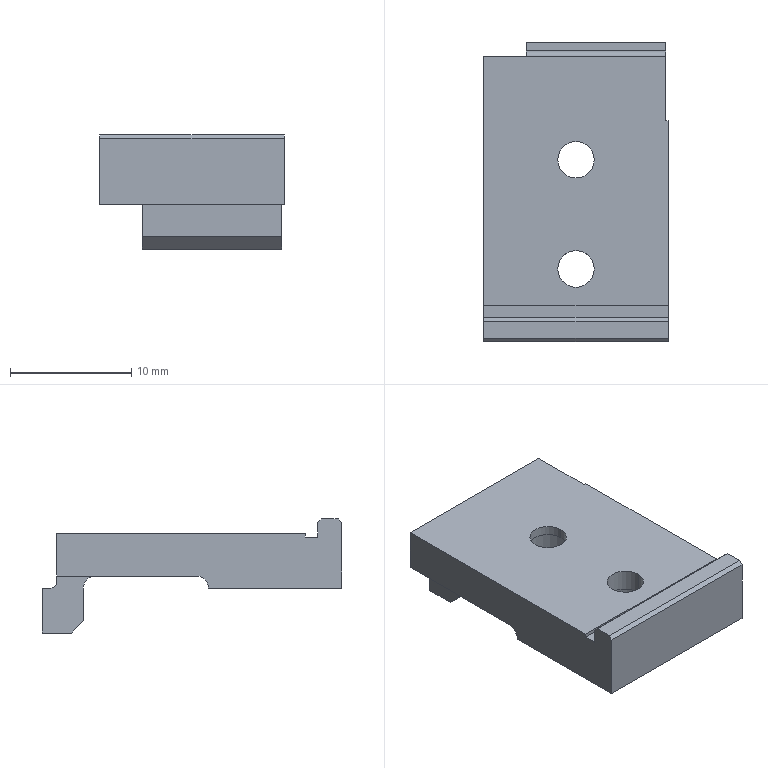Part | NX | 1 solid | 34 faces | box 15.2 x 24.7 x 9.4 mm | volume 1490 mm3 | plane 23 | cylinder 11 | commonest cylinder face diameters 3 x4 5 x4 2 x2 1 x1
STEP:
#1=CARTESIAN_POINT('',(-15.2,-12.7,1.));
#2=VERTEX_POINT('',#1);
#3=CARTESIAN_POINT('',(-15.2,-1.2,1.));
#4=VERTEX_POINT('',#3);
#5=CARTESIAN_POINT('',(-15.2,0.,1.));
#6=DIRECTION('',(0.,1.,0.));
#7=VECTOR('',#6,1000.);
#8=LINE('',#5,#7);
#9=EDGE_CURVE('',#2,#4,#8,.T.);
#10=ORIENTED_EDGE('',*,*,#9,.F.);
#11=CARTESIAN_POINT('',(-15.2,-13.7,0.));
#12=VERTEX_POINT('',#11);
#13=CARTESIAN_POINT('',(-15.2,-12.7,0.));
#14=DIRECTION('',(1.,0.,0.));
#15=DIRECTION('',(0.,-1.,0.));
#16=AXIS2_PLACEMENT_3D('',#13,#14,#15);
#17=CIRCLE('',#16,1.);
#18=EDGE_CURVE('',#2,#12,#17,.T.);
#19=ORIENTED_EDGE('',*,*,#18,.T.);
#20=CARTESIAN_POINT('',(-15.2,-24.7,0.));
#21=VERTEX_POINT('',#20);
#22=CARTESIAN_POINT('',(-15.2,0.,0.));
#23=DIRECTION('',(0.,1.,0.));
#24=VECTOR('',#23,1000.);
#25=LINE('',#22,#24);
#26=EDGE_CURVE('',#21,#12,#25,.T.);
#27=ORIENTED_EDGE('',*,*,#26,.F.);
#28=CARTESIAN_POINT('',(-15.2,-24.7,5.4));
#29=VERTEX_POINT('',#28);
#30=CARTESIAN_POINT('',(-15.2,-24.7,0.));
#31=DIRECTION('',(0.,0.,-1.));
#32=VECTOR('',#31,1000.);
#33=LINE('',#30,#32);
#34=EDGE_CURVE('',#29,#21,#33,.T.);
#35=ORIENTED_EDGE('',*,*,#34,.F.);
#36=CARTESIAN_POINT('',(-15.2,-24.4,5.7));
#37=VERTEX_POINT('',#36);
#38=CARTESIAN_POINT('',(-15.2,0.,30.1));
#39=DIRECTION('',(0.,0.7071,0.7071));
#40=VECTOR('',#39,1000.);
#41=LINE('',#38,#40);
#42=EDGE_CURVE('',#29,#37,#41,.T.);
#43=ORIENTED_EDGE('',*,*,#42,.T.);
#44=CARTESIAN_POINT('',(-15.2,-23.,5.7));
#45=VERTEX_POINT('',#44);
#46=CARTESIAN_POINT('',(-15.2,0.,5.7));
#47=DIRECTION('',(0.,1.,0.));
#48=VECTOR('',#47,1000.);
#49=LINE('',#46,#48);
#50=EDGE_CURVE('',#37,#45,#49,.T.);
#51=ORIENTED_EDGE('',*,*,#50,.T.);
#52=CARTESIAN_POINT('',(-15.2,-22.7,5.4));
#53=VERTEX_POINT('',#52);
#54=CARTESIAN_POINT('',(-15.2,0.,-17.3));
#55=DIRECTION('',(0.,-0.7071,0.7071));
#56=VECTOR('',#55,1000.);
#57=LINE('',#54,#56);
#58=EDGE_CURVE('',#53,#45,#57,.T.);
#59=ORIENTED_EDGE('',*,*,#58,.F.);
#60=CARTESIAN_POINT('',(-15.2,-22.7,4.2));
#61=VERTEX_POINT('',#60);
#62=CARTESIAN_POINT('',(-15.2,-22.7,0.));
#63=DIRECTION('',(0.,0.,-1.));
#64=VECTOR('',#63,1000.);
#65=LINE('',#62,#64);
#66=EDGE_CURVE('',#53,#61,#65,.T.);
#67=ORIENTED_EDGE('',*,*,#66,.T.);
#68=CARTESIAN_POINT('',(-15.2,-21.7,4.2));
#69=VERTEX_POINT('',#68);
#70=CARTESIAN_POINT('',(-15.2,0.,4.2));
#71=DIRECTION('',(0.,-1.,0.));
#72=VECTOR('',#71,1000.);
#73=LINE('',#70,#72);
#74=EDGE_CURVE('',#69,#61,#73,.T.);
#75=ORIENTED_EDGE('',*,*,#74,.F.);
#76=CARTESIAN_POINT('',(-15.2,-21.7,4.5));
#77=VERTEX_POINT('',#76);
#78=CARTESIAN_POINT('',(-15.2,-21.7,0.));
#79=DIRECTION('',(0.,0.,-1.));
#80=VECTOR('',#79,1000.);
#81=LINE('',#78,#80);
#82=EDGE_CURVE('',#77,#69,#81,.T.);
#83=ORIENTED_EDGE('',*,*,#82,.F.);
#84=CARTESIAN_POINT('',(-15.2,-1.2,4.5));
#85=VERTEX_POINT('',#84);
#86=CARTESIAN_POINT('',(-15.2,0.,4.5));
#87=DIRECTION('',(0.,-1.,0.));
#88=VECTOR('',#87,1000.);
#89=LINE('',#86,#88);
#90=EDGE_CURVE('',#85,#77,#89,.T.);
#91=ORIENTED_EDGE('',*,*,#90,.F.);
#92=CARTESIAN_POINT('',(-15.2,-1.2,0.));
#93=DIRECTION('',(0.,0.,1.));
#94=VECTOR('',#93,1000.);
#95=LINE('',#92,#94);
#96=EDGE_CURVE('',#4,#85,#95,.T.);
#97=ORIENTED_EDGE('',*,*,#96,.F.);
#98=EDGE_LOOP('',(#10,#19,#27,#35,#43,#51,#59,#67,#75,#83,#91,#97));
#99=FACE_BOUND('',#98,.T.);
#100=CARTESIAN_POINT('',(-15.2,0.,0.));
#101=DIRECTION('',(1.,0.,0.));
#102=DIRECTION('',(0.,1.,0.));
#103=AXIS2_PLACEMENT_3D('',#100,#101,#102);
#104=PLANE('',#103);
#105=ADVANCED_FACE('',(#99),#104,.F.);
#106=CARTESIAN_POINT('',(0.,-21.7,4.5));
#107=VERTEX_POINT('',#106);
#108=CARTESIAN_POINT('',(0.,-6.5,4.5));
#109=VERTEX_POINT('',#108);
#110=CARTESIAN_POINT('',(0.,0.,4.5));
#111=DIRECTION('',(0.,1.,0.));
#112=VECTOR('',#111,1000.);
#113=LINE('',#110,#112);
#114=EDGE_CURVE('',#107,#109,#113,.T.);
#115=ORIENTED_EDGE('',*,*,#114,.F.);
#116=CARTESIAN_POINT('',(0.,-21.7,4.2));
#117=VERTEX_POINT('',#116);
#118=CARTESIAN_POINT('',(0.,-21.7,0.));
#119=DIRECTION('',(0.,0.,1.));
#120=VECTOR('',#119,1000.);
#121=LINE('',#118,#120);
#122=EDGE_CURVE('',#117,#107,#121,.T.);
#123=ORIENTED_EDGE('',*,*,#122,.F.);
#124=CARTESIAN_POINT('',(0.,-22.7,4.2));
#125=VERTEX_POINT('',#124);
#126=CARTESIAN_POINT('',(0.,0.,4.2));
#127=DIRECTION('',(0.,1.,0.));
#128=VECTOR('',#127,1000.);
#129=LINE('',#126,#128);
#130=EDGE_CURVE('',#125,#117,#129,.T.);
#131=ORIENTED_EDGE('',*,*,#130,.F.);
#132=CARTESIAN_POINT('',(0.,-22.7,5.4));
#133=VERTEX_POINT('',#132);
#134=CARTESIAN_POINT('',(0.,-22.7,0.));
#135=DIRECTION('',(0.,0.,1.));
#136=VECTOR('',#135,1000.);
#137=LINE('',#134,#136);
#138=EDGE_CURVE('',#125,#133,#137,.T.);
#139=ORIENTED_EDGE('',*,*,#138,.T.);
#140=CARTESIAN_POINT('',(0.,-23.,5.7));
#141=VERTEX_POINT('',#140);
#142=CARTESIAN_POINT('',(0.,0.,-17.3));
#143=DIRECTION('',(0.,0.7071,-0.7071));
#144=VECTOR('',#143,1000.);
#145=LINE('',#142,#144);
#146=EDGE_CURVE('',#141,#133,#145,.T.);
#147=ORIENTED_EDGE('',*,*,#146,.F.);
#148=CARTESIAN_POINT('',(0.,-24.4,5.7));
#149=VERTEX_POINT('',#148);
#150=CARTESIAN_POINT('',(0.,0.,5.7));
#151=DIRECTION('',(0.,-1.,0.));
#152=VECTOR('',#151,1000.);
#153=LINE('',#150,#152);
#154=EDGE_CURVE('',#141,#149,#153,.T.);
#155=ORIENTED_EDGE('',*,*,#154,.T.);
#156=CARTESIAN_POINT('',(0.,-24.7,5.4));
#157=VERTEX_POINT('',#156);
#158=CARTESIAN_POINT('',(0.,0.,30.1));
#159=DIRECTION('',(0.,-0.7071,-0.7071));
#160=VECTOR('',#159,1000.);
#161=LINE('',#158,#160);
#162=EDGE_CURVE('',#149,#157,#161,.T.);
#163=ORIENTED_EDGE('',*,*,#162,.T.);
#164=CARTESIAN_POINT('',(0.,-24.7,0.));
#165=VERTEX_POINT('',#164);
#166=CARTESIAN_POINT('',(0.,-24.7,0.));
#167=DIRECTION('',(0.,0.,1.));
#168=VECTOR('',#167,1000.);
#169=LINE('',#166,#168);
#170=EDGE_CURVE('',#165,#157,#169,.T.);
#171=ORIENTED_EDGE('',*,*,#170,.F.);
#172=CARTESIAN_POINT('',(0.,-13.7,0.));
#173=VERTEX_POINT('',#172);
#174=CARTESIAN_POINT('',(0.,0.,0.));
#175=DIRECTION('',(0.,-1.,0.));
#176=VECTOR('',#175,1000.);
#177=LINE('',#174,#176);
#178=EDGE_CURVE('',#173,#165,#177,.T.);
#179=ORIENTED_EDGE('',*,*,#178,.F.);
#180=CARTESIAN_POINT('',(0.,-12.7,1.));
#181=VERTEX_POINT('',#180);
#182=CARTESIAN_POINT('',(0.,-12.7,0.));
#183=DIRECTION('',(1.,0.,0.));
#184=DIRECTION('',(0.,-1.,0.));
#185=AXIS2_PLACEMENT_3D('',#182,#183,#184);
#186=CIRCLE('',#185,1.);
#187=EDGE_CURVE('',#181,#173,#186,.T.);
#188=ORIENTED_EDGE('',*,*,#187,.F.);
#189=CARTESIAN_POINT('',(0.,-6.5,1.));
#190=VERTEX_POINT('',#189);
#191=CARTESIAN_POINT('',(0.,0.,1.));
#192=DIRECTION('',(0.,-1.,0.));
#193=VECTOR('',#192,1000.);
#194=LINE('',#191,#193);
#195=EDGE_CURVE('',#190,#181,#194,.T.);
#196=ORIENTED_EDGE('',*,*,#195,.F.);
#197=CARTESIAN_POINT('',(0.,-6.5,0.));
#198=DIRECTION('',(0.,0.,-1.));
#199=VECTOR('',#198,1000.);
#200=LINE('',#197,#199);
#201=EDGE_CURVE('',#109,#190,#200,.T.);
#202=ORIENTED_EDGE('',*,*,#201,.F.);
#203=EDGE_LOOP('',(#115,#123,#131,#139,#147,#155,#163,#171,#179,#188,#196,#202));
#204=FACE_BOUND('',#203,.T.);
#205=CARTESIAN_POINT('',(0.,-24.7,0.));
#206=DIRECTION('',(-1.,0.,0.));
#207=DIRECTION('',(0.,0.,1.));
#208=AXIS2_PLACEMENT_3D('',#205,#206,#207);
#209=PLANE('',#208);
#210=ADVANCED_FACE('',(#204),#209,.F.);
#211=CARTESIAN_POINT('',(-5.1,-18.7,2.7));
#212=VERTEX_POINT('',#211);
#213=CARTESIAN_POINT('',(-10.1,-18.7,2.7));
#214=VERTEX_POINT('',#213);
#215=CARTESIAN_POINT('',(-7.6,-18.7,2.7));
#216=DIRECTION('',(0.,0.,-1.));
#217=DIRECTION('',(-1.,0.,0.));
#218=AXIS2_PLACEMENT_3D('',#215,#216,#217);
#219=CIRCLE('',#218,2.5);
#220=EDGE_CURVE('',#212,#214,#219,.T.);
#221=ORIENTED_EDGE('',*,*,#220,.T.);
#222=CARTESIAN_POINT('',(-7.6,-18.7,2.7));
#223=DIRECTION('',(0.,0.,-1.));
#224=DIRECTION('',(-1.,0.,0.));
#225=AXIS2_PLACEMENT_3D('',#222,#223,#224);
#226=CIRCLE('',#225,2.5);
#227=EDGE_CURVE('',#214,#212,#226,.T.);
#228=ORIENTED_EDGE('',*,*,#227,.T.);
#229=EDGE_LOOP('',(#221,#228));
#230=FACE_BOUND('',#229,.T.);
#231=CARTESIAN_POINT('',(-9.1,-18.7,2.7));
#232=VERTEX_POINT('',#231);
#233=CARTESIAN_POINT('',(-6.1,-18.7,2.7));
#234=VERTEX_POINT('',#233);
#235=CARTESIAN_POINT('',(-7.6,-18.7,2.7));
#236=DIRECTION('',(0.,0.,-1.));
#237=DIRECTION('',(-1.,0.,0.));
#238=AXIS2_PLACEMENT_3D('',#235,#236,#237);
#239=CIRCLE('',#238,1.5);
#240=EDGE_CURVE('',#232,#234,#239,.T.);
#241=ORIENTED_EDGE('',*,*,#240,.F.);
#242=CARTESIAN_POINT('',(-7.6,-18.7,2.7));
#243=DIRECTION('',(0.,0.,-1.));
#244=DIRECTION('',(-1.,0.,0.));
#245=AXIS2_PLACEMENT_3D('',#242,#243,#244);
#246=CIRCLE('',#245,1.5);
#247=EDGE_CURVE('',#234,#232,#246,.T.);
#248=ORIENTED_EDGE('',*,*,#247,.F.);
#249=EDGE_LOOP('',(#241,#248));
#250=FACE_BOUND('',#249,.T.);
#251=CARTESIAN_POINT('',(-11.486,-5.492,2.7));
#252=DIRECTION('',(0.,0.,-1.));
#253=DIRECTION('',(0.,-1.,0.));
#254=AXIS2_PLACEMENT_3D('',#251,#252,#253);
#255=PLANE('',#254);
#256=ADVANCED_FACE('',(#230,#250),#255,.T.);
#257=CARTESIAN_POINT('',(-0.2,-1.2,4.5));
#258=VERTEX_POINT('',#257);
#259=CARTESIAN_POINT('',(-0.2,-6.5,4.5));
#260=VERTEX_POINT('',#259);
#261=CARTESIAN_POINT('',(-0.2,0.,4.5));
#262=DIRECTION('',(0.,-1.,0.));
#263=VECTOR('',#262,1000.);
#264=LINE('',#261,#263);
#265=EDGE_CURVE('',#258,#260,#264,.T.);
#266=ORIENTED_EDGE('',*,*,#265,.F.);
#267=CARTESIAN_POINT('',(0.,-1.2,4.5));
#268=DIRECTION('',(1.,0.,0.));
#269=VECTOR('',#268,1000.);
#270=LINE('',#267,#269);
#271=EDGE_CURVE('',#85,#258,#270,.T.);
#272=ORIENTED_EDGE('',*,*,#271,.F.);
#273=ORIENTED_EDGE('',*,*,#90,.T.);
#274=CARTESIAN_POINT('',(0.,-21.7,4.5));
#275=DIRECTION('',(-1.,0.,0.));
#276=VECTOR('',#275,1000.);
#277=LINE('',#274,#276);
#278=EDGE_CURVE('',#107,#77,#277,.T.);
#279=ORIENTED_EDGE('',*,*,#278,.F.);
#280=ORIENTED_EDGE('',*,*,#114,.T.);
#281=CARTESIAN_POINT('',(0.,-6.5,4.5));
#282=DIRECTION('',(1.,0.,0.));
#283=VECTOR('',#282,1000.);
#284=LINE('',#281,#283);
#285=EDGE_CURVE('',#260,#109,#284,.T.);
#286=ORIENTED_EDGE('',*,*,#285,.F.);
#287=EDGE_LOOP('',(#266,#272,#273,#279,#280,#286));
#288=FACE_BOUND('',#287,.T.);
#289=CARTESIAN_POINT('',(-6.1,-9.7,4.5));
#290=VERTEX_POINT('',#289);
#291=CARTESIAN_POINT('',(-9.1,-9.7,4.5));
#292=VERTEX_POINT('',#291);
#293=CARTESIAN_POINT('',(-7.6,-9.7,4.5));
#294=DIRECTION('',(0.,0.,-1.));
#295=DIRECTION('',(-1.,0.,0.));
#296=AXIS2_PLACEMENT_3D('',#293,#294,#295);
#297=CIRCLE('',#296,1.5);
#298=EDGE_CURVE('',#290,#292,#297,.T.);
#299=ORIENTED_EDGE('',*,*,#298,.T.);
#300=CARTESIAN_POINT('',(-7.6,-9.7,4.5));
#301=DIRECTION('',(0.,0.,-1.));
#302=DIRECTION('',(-1.,0.,0.));
#303=AXIS2_PLACEMENT_3D('',#300,#301,#302);
#304=CIRCLE('',#303,1.5);
#305=EDGE_CURVE('',#292,#290,#304,.T.);
#306=ORIENTED_EDGE('',*,*,#305,.T.);
#307=EDGE_LOOP('',(#299,#306));
#308=FACE_BOUND('',#307,.T.);
#309=CARTESIAN_POINT('',(-9.1,-18.7,4.5));
#310=VERTEX_POINT('',#309);
#311=CARTESIAN_POINT('',(-6.1,-18.7,4.5));
#312=VERTEX_POINT('',#311);
#313=CARTESIAN_POINT('',(-7.6,-18.7,4.5));
#314=DIRECTION('',(0.,0.,-1.));
#315=DIRECTION('',(-1.,0.,0.));
#316=AXIS2_PLACEMENT_3D('',#313,#314,#315);
#317=CIRCLE('',#316,1.5);
#318=EDGE_CURVE('',#310,#312,#317,.T.);
#319=ORIENTED_EDGE('',*,*,#318,.T.);
#320=CARTESIAN_POINT('',(-7.6,-18.7,4.5));
#321=DIRECTION('',(0.,0.,-1.));
#322=DIRECTION('',(-1.,0.,0.));
#323=AXIS2_PLACEMENT_3D('',#320,#321,#322);
#324=CIRCLE('',#323,1.5);
#325=EDGE_CURVE('',#312,#310,#324,.T.);
#326=ORIENTED_EDGE('',*,*,#325,.T.);
#327=EDGE_LOOP('',(#319,#326));
#328=FACE_BOUND('',#327,.T.);
#329=CARTESIAN_POINT('',(0.,0.,4.5));
#330=DIRECTION('',(0.,0.,1.));
#331=DIRECTION('',(1.,0.,0.));
#332=AXIS2_PLACEMENT_3D('',#329,#330,#331);
#333=PLANE('',#332);
#334=ADVANCED_FACE('',(#288,#308,#328),#333,.T.);
#335=CARTESIAN_POINT('',(-0.2,-3.4,-2.7));
#336=VERTEX_POINT('',#335);
#337=CARTESIAN_POINT('',(-0.2,-3.4,0.));
#338=VERTEX_POINT('',#337);
#339=CARTESIAN_POINT('',(-0.2,-3.4,0.));
#340=DIRECTION('',(0.,0.,1.));
#341=VECTOR('',#340,1000.);
#342=LINE('',#339,#341);
#343=EDGE_CURVE('',#336,#338,#342,.T.);
#344=ORIENTED_EDGE('',*,*,#343,.F.);
#345=CARTESIAN_POINT('',(-0.2,-2.4,-3.7));
#346=VERTEX_POINT('',#345);
#347=CARTESIAN_POINT('',(-0.2,-6.1,0.));
#348=DIRECTION('',(0.,0.7071,-0.7071));
#349=VECTOR('',#348,1000.);
#350=LINE('',#347,#349);
#351=EDGE_CURVE('',#336,#346,#350,.T.);
#352=ORIENTED_EDGE('',*,*,#351,.T.);
#353=CARTESIAN_POINT('',(-0.2,0.,-3.7));
#354=VERTEX_POINT('',#353);
#355=CARTESIAN_POINT('',(-0.2,0.,-3.7));
#356=DIRECTION('',(0.,-1.,0.));
#357=VECTOR('',#356,1000.);
#358=LINE('',#355,#357);
#359=EDGE_CURVE('',#354,#346,#358,.T.);
#360=ORIENTED_EDGE('',*,*,#359,.F.);
#361=CARTESIAN_POINT('',(-0.2,0.,0.));
#362=VERTEX_POINT('',#361);
#363=CARTESIAN_POINT('',(-0.2,0.,0.));
#364=DIRECTION('',(0.,0.,-1.));
#365=VECTOR('',#364,1000.);
#366=LINE('',#363,#365);
#367=EDGE_CURVE('',#362,#354,#366,.T.);
#368=ORIENTED_EDGE('',*,*,#367,.F.);
#369=CARTESIAN_POINT('',(-0.2,-0.7,0.));
#370=VERTEX_POINT('',#369);
#371=CARTESIAN_POINT('',(-0.2,0.,0.));
#372=DIRECTION('',(0.,-1.,0.));
#373=VECTOR('',#372,1000.);
#374=LINE('',#371,#373);
#375=EDGE_CURVE('',#362,#370,#374,.T.);
#376=ORIENTED_EDGE('',*,*,#375,.T.);
#377=CARTESIAN_POINT('',(-0.2,-1.2,0.5));
#378=VERTEX_POINT('',#377);
#379=CARTESIAN_POINT('',(-0.2,-0.7,0.5));
#380=DIRECTION('',(-1.,0.,0.));
#381=DIRECTION('',(0.,1.,0.));
#382=AXIS2_PLACEMENT_3D('',#379,#380,#381);
#383=CIRCLE('',#382,0.5);
#384=EDGE_CURVE('',#370,#378,#383,.T.);
#385=ORIENTED_EDGE('',*,*,#384,.T.);
#386=CARTESIAN_POINT('',(-0.2,-1.2,0.));
#387=DIRECTION('',(0.,0.,1.));
#388=VECTOR('',#387,1000.);
#389=LINE('',#386,#388);
#390=EDGE_CURVE('',#378,#258,#389,.T.);
#391=ORIENTED_EDGE('',*,*,#390,.T.);
#392=ORIENTED_EDGE('',*,*,#265,.T.);
#393=CARTESIAN_POINT('',(-0.2,-6.5,1.));
#394=VERTEX_POINT('',#393);
#395=CARTESIAN_POINT('',(-0.2,-6.5,0.));
#396=DIRECTION('',(0.,0.,1.));
#397=VECTOR('',#396,1000.);
#398=LINE('',#395,#397);
#399=EDGE_CURVE('',#394,#260,#398,.T.);
#400=ORIENTED_EDGE('',*,*,#399,.F.);
#401=CARTESIAN_POINT('',(-0.2,-4.4,1.));
#402=VERTEX_POINT('',#401);
#403=CARTESIAN_POINT('',(-0.2,0.,1.));
#404=DIRECTION('',(0.,1.,0.));
#405=VECTOR('',#404,1000.);
#406=LINE('',#403,#405);
#407=EDGE_CURVE('',#394,#402,#406,.T.);
#408=ORIENTED_EDGE('',*,*,#407,.T.);
#409=CARTESIAN_POINT('',(-0.2,-4.4,0.));
#410=DIRECTION('',(-1.,0.,0.));
#411=DIRECTION('',(0.,1.,0.));
#412=AXIS2_PLACEMENT_3D('',#409,#410,#411);
#413=CIRCLE('',#412,1.);
#414=EDGE_CURVE('',#402,#338,#413,.T.);
#415=ORIENTED_EDGE('',*,*,#414,.T.);
#416=EDGE_LOOP('',(#344,#352,#360,#368,#376,#385,#391,#392,#400,#408,#415));
#417=FACE_BOUND('',#416,.T.);
#418=CARTESIAN_POINT('',(-0.2,-6.5,2.));
#419=DIRECTION('',(1.,0.,0.));
#420=DIRECTION('',(0.,1.,0.));
#421=AXIS2_PLACEMENT_3D('',#418,#419,#420);
#422=PLANE('',#421);
#423=ADVANCED_FACE('',(#417),#422,.T.);
#424=ORIENTED_EDGE('',*,*,#82,.T.);
#425=CARTESIAN_POINT('',(0.,-21.7,4.2));
#426=DIRECTION('',(1.,0.,0.));
#427=VECTOR('',#426,1000.);
#428=LINE('',#425,#427);
#429=EDGE_CURVE('',#69,#117,#428,.T.);
#430=ORIENTED_EDGE('',*,*,#429,.T.);
#431=ORIENTED_EDGE('',*,*,#122,.T.);
#432=ORIENTED_EDGE('',*,*,#278,.T.);
#433=EDGE_LOOP('',(#424,#430,#431,#432));
#434=FACE_BOUND('',#433,.T.);
#435=CARTESIAN_POINT('',(0.,-21.7,2.));
#436=DIRECTION('',(0.,-1.,0.));
#437=DIRECTION('',(0.,0.,-1.));
#438=AXIS2_PLACEMENT_3D('',#435,#436,#437);
#439=PLANE('',#438);
#440=ADVANCED_FACE('',(#434),#439,.T.);
#441=CARTESIAN_POINT('',(-11.7,-3.4,0.));
#442=VERTEX_POINT('',#441);
#443=CARTESIAN_POINT('',(-11.7,-3.4,-2.7));
#444=VERTEX_POINT('',#443);
#445=CARTESIAN_POINT('',(-11.7,-3.4,0.));
#446=DIRECTION('',(0.,0.,-1.));
#447=VECTOR('',#446,1000.);
#448=LINE('',#445,#447);
#449=EDGE_CURVE('',#442,#444,#448,.T.);
#450=ORIENTED_EDGE('',*,*,#449,.F.);
#451=CARTESIAN_POINT('',(-11.7,-4.4,1.));
#452=VERTEX_POINT('',#451);
#453=CARTESIAN_POINT('',(-11.7,-4.4,0.));
#454=DIRECTION('',(-1.,0.,0.));
#455=DIRECTION('',(0.,1.,0.));
#456=AXIS2_PLACEMENT_3D('',#453,#454,#455);
#457=CIRCLE('',#456,1.);
#458=EDGE_CURVE('',#452,#442,#457,.T.);
#459=ORIENTED_EDGE('',*,*,#458,.F.);
#460=CARTESIAN_POINT('',(-11.7,-1.2,1.));
#461=VERTEX_POINT('',#460);
#462=CARTESIAN_POINT('',(-11.7,0.,1.));
#463=DIRECTION('',(0.,1.,0.));
#464=VECTOR('',#463,1000.);
#465=LINE('',#462,#464);
#466=EDGE_CURVE('',#452,#461,#465,.T.);
#467=ORIENTED_EDGE('',*,*,#466,.T.);
#468=CARTESIAN_POINT('',(-11.7,-1.2,0.5));
#469=VERTEX_POINT('',#468);
#470=CARTESIAN_POINT('',(-11.7,-1.2,0.));
#471=DIRECTION('',(0.,0.,1.));
#472=VECTOR('',#471,1000.);
#473=LINE('',#470,#472);
#474=EDGE_CURVE('',#469,#461,#473,.T.);
#475=ORIENTED_EDGE('',*,*,#474,.F.);
#476=CARTESIAN_POINT('',(-11.7,-0.7,0.));
#477=VERTEX_POINT('',#476);
#478=CARTESIAN_POINT('',(-11.7,-0.7,0.5));
#479=DIRECTION('',(-1.,0.,0.));
#480=DIRECTION('',(0.,1.,0.));
#481=AXIS2_PLACEMENT_3D('',#478,#479,#480);
#482=CIRCLE('',#481,0.5);
#483=EDGE_CURVE('',#477,#469,#482,.T.);
#484=ORIENTED_EDGE('',*,*,#483,.F.);
#485=CARTESIAN_POINT('',(-11.7,0.,0.));
#486=VERTEX_POINT('',#485);
#487=CARTESIAN_POINT('',(-11.7,0.,0.));
#488=DIRECTION('',(0.,-1.,0.));
#489=VECTOR('',#488,1000.);
#490=LINE('',#487,#489);
#491=EDGE_CURVE('',#486,#477,#490,.T.);
#492=ORIENTED_EDGE('',*,*,#491,.F.);
#493=CARTESIAN_POINT('',(-11.7,0.,-3.7));
#494=VERTEX_POINT('',#493);
#495=CARTESIAN_POINT('',(-11.7,0.,0.));
#496=DIRECTION('',(0.,0.,-1.));
#497=VECTOR('',#496,1000.);
#498=LINE('',#495,#497);
#499=EDGE_CURVE('',#486,#494,#498,.T.);
#500=ORIENTED_EDGE('',*,*,#499,.T.);
#501=CARTESIAN_POINT('',(-11.7,-2.4,-3.7));
#502=VERTEX_POINT('',#501);
#503=CARTESIAN_POINT('',(-11.7,0.,-3.7));
#504=DIRECTION('',(0.,1.,0.));
#505=VECTOR('',#504,1000.);
#506=LINE('',#503,#505);
#507=EDGE_CURVE('',#502,#494,#506,.T.);
#508=ORIENTED_EDGE('',*,*,#507,.F.);
#509=CARTESIAN_POINT('',(-11.7,-6.1,0.));
#510=DIRECTION('',(0.,0.7071,-0.7071));
#511=VECTOR('',#510,1000.);
#512=LINE('',#509,#511);
#513=EDGE_CURVE('',#444,#502,#512,.T.);
#514=ORIENTED_EDGE('',*,*,#513,.F.);
#515=EDGE_LOOP('',(#450,#459,#467,#475,#484,#492,#500,#508,#514));
#516=FACE_BOUND('',#515,.T.);
#517=CARTESIAN_POINT('',(-11.7,-1.2,0.));
#518=DIRECTION('',(1.,0.,0.));
#519=DIRECTION('',(0.,1.,0.));
#520=AXIS2_PLACEMENT_3D('',#517,#518,#519);
#521=PLANE('',#520);
#522=ADVANCED_FACE('',(#516),#521,.F.);
#523=CARTESIAN_POINT('',(0.,-6.5,1.));
#524=DIRECTION('',(-1.,0.,0.));
#525=VECTOR('',#524,1000.);
#526=LINE('',#523,#525);
#527=EDGE_CURVE('',#190,#394,#526,.T.);
#528=ORIENTED_EDGE('',*,*,#527,.T.);
#529=ORIENTED_EDGE('',*,*,#399,.T.);
#530=ORIENTED_EDGE('',*,*,#285,.T.);
#531=ORIENTED_EDGE('',*,*,#201,.T.);
#532=EDGE_LOOP('',(#528,#529,#530,#531));
#533=FACE_BOUND('',#532,.T.);
#534=CARTESIAN_POINT('',(0.,-6.5,2.));
#535=DIRECTION('',(0.,1.,0.));
#536=DIRECTION('',(1.,0.,0.));
#537=AXIS2_PLACEMENT_3D('',#534,#535,#536);
#538=PLANE('',#537);
#539=ADVANCED_FACE('',(#533),#538,.T.);
#540=CARTESIAN_POINT('',(0.,-13.7,0.));
#541=DIRECTION('',(1.,0.,0.));
#542=VECTOR('',#541,1000.);
#543=LINE('',#540,#542);
#544=EDGE_CURVE('',#12,#173,#543,.T.);
#545=ORIENTED_EDGE('',*,*,#544,.T.);
#546=ORIENTED_EDGE('',*,*,#178,.T.);
#547=CARTESIAN_POINT('',(0.,-24.7,0.));
#548=DIRECTION('',(1.,0.,0.));
#549=VECTOR('',#548,1000.);
#550=LINE('',#547,#549);
#551=EDGE_CURVE('',#21,#165,#550,.T.);
#552=ORIENTED_EDGE('',*,*,#551,.F.);
#553=ORIENTED_EDGE('',*,*,#26,.T.);
#554=EDGE_LOOP('',(#545,#546,#552,#553));
#555=FACE_BOUND('',#554,.T.);
#556=CARTESIAN_POINT('',(-10.1,-18.7,0.));
#557=VERTEX_POINT('',#556);
#558=CARTESIAN_POINT('',(-5.1,-18.7,0.));
#559=VERTEX_POINT('',#558);
#560=CARTESIAN_POINT('',(-7.6,-18.7,0.));
#561=DIRECTION('',(0.,0.,-1.));
#562=DIRECTION('',(-1.,0.,0.));
#563=AXIS2_PLACEMENT_3D('',#560,#561,#562);
#564=CIRCLE('',#563,2.5);
#565=EDGE_CURVE('',#557,#559,#564,.T.);
#566=ORIENTED_EDGE('',*,*,#565,.F.);
#567=CARTESIAN_POINT('',(-7.6,-18.7,0.));
#568=DIRECTION('',(0.,0.,-1.));
#569=DIRECTION('',(-1.,0.,0.));
#570=AXIS2_PLACEMENT_3D('',#567,#568,#569);
#571=CIRCLE('',#570,2.5);
#572=EDGE_CURVE('',#559,#557,#571,.T.);
#573=ORIENTED_EDGE('',*,*,#572,.F.);
#574=EDGE_LOOP('',(#566,#573));
#575=FACE_BOUND('',#574,.T.);
#576=CARTESIAN_POINT('',(-11.977,-15.053,0.));
#577=DIRECTION('',(0.,0.,-1.));
#578=DIRECTION('',(0.,-1.,0.));
#579=AXIS2_PLACEMENT_3D('',#576,#577,#578);
#580=PLANE('',#579);
#581=ADVANCED_FACE('',(#555,#575),#580,.T.);
#582=ORIENTED_EDGE('',*,*,#375,.F.);
#583=CARTESIAN_POINT('',(0.,0.,0.));
#584=DIRECTION('',(1.,0.,0.));
#585=VECTOR('',#584,1000.);
#586=LINE('',#583,#585);
#587=EDGE_CURVE('',#486,#362,#586,.T.);
#588=ORIENTED_EDGE('',*,*,#587,.F.);
#589=ORIENTED_EDGE('',*,*,#491,.T.);
#590=CARTESIAN_POINT('',(0.,-0.7,0.));
#591=DIRECTION('',(-1.,0.,0.));
#592=VECTOR('',#591,1000.);
#593=LINE('',#590,#592);
#594=EDGE_CURVE('',#370,#477,#593,.T.);
#595=ORIENTED_EDGE('',*,*,#594,.F.);
#596=EDGE_LOOP('',(#582,#588,#589,#595));
#597=FACE_BOUND('',#596,.T.);
#598=CARTESIAN_POINT('',(-15.2,-1.2,0.));
#599=DIRECTION('',(0.,0.,1.));
#600=DIRECTION('',(1.,0.,0.));
#601=AXIS2_PLACEMENT_3D('',#598,#599,#600);
#602=PLANE('',#601);
#603=ADVANCED_FACE('',(#597),#602,.T.);
#604=CARTESIAN_POINT('',(0.,0.,-3.7));
#605=DIRECTION('',(1.,0.,0.));
#606=VECTOR('',#605,1000.);
#607=LINE('',#604,#606);
#608=EDGE_CURVE('',#494,#354,#607,.T.);
#609=ORIENTED_EDGE('',*,*,#608,.F.);
#610=ORIENTED_EDGE('',*,*,#499,.F.);
#611=ORIENTED_EDGE('',*,*,#587,.T.);
#612=ORIENTED_EDGE('',*,*,#367,.T.);
#613=EDGE_LOOP('',(#609,#610,#611,#612));
#614=FACE_BOUND('',#613,.T.);
#615=CARTESIAN_POINT('',(0.,0.,0.));
#616=DIRECTION('',(0.,-1.,0.));
#617=DIRECTION('',(0.,0.,-1.));
#618=AXIS2_PLACEMENT_3D('',#615,#616,#617);
#619=PLANE('',#618);
#620=ADVANCED_FACE('',(#614),#619,.F.);
#621=CARTESIAN_POINT('',(0.,-2.4,-3.7));
#622=DIRECTION('',(1.,0.,0.));
#623=VECTOR('',#622,1000.);
#624=LINE('',#621,#623);
#625=EDGE_CURVE('',#502,#346,#624,.T.);
#626=ORIENTED_EDGE('',*,*,#625,.F.);
#627=ORIENTED_EDGE('',*,*,#507,.T.);
#628=ORIENTED_EDGE('',*,*,#608,.T.);
#629=ORIENTED_EDGE('',*,*,#359,.T.);
#630=EDGE_LOOP('',(#626,#627,#628,#629));
#631=FACE_BOUND('',#630,.T.);
#632=CARTESIAN_POINT('',(0.,0.,-3.7));
#633=DIRECTION('',(0.,0.,1.));
#634=DIRECTION('',(1.,0.,0.));
#635=AXIS2_PLACEMENT_3D('',#632,#633,#634);
#636=PLANE('',#635);
#637=ADVANCED_FACE('',(#631),#636,.F.);
#638=CARTESIAN_POINT('',(0.,-22.7,4.2));
#639=DIRECTION('',(1.,0.,0.));
#640=VECTOR('',#639,1000.);
#641=LINE('',#638,#640);
#642=EDGE_CURVE('',#61,#125,#641,.T.);
#643=ORIENTED_EDGE('',*,*,#642,.T.);
#644=ORIENTED_EDGE('',*,*,#130,.T.);
#645=ORIENTED_EDGE('',*,*,#429,.F.);
#646=ORIENTED_EDGE('',*,*,#74,.T.);
#647=EDGE_LOOP('',(#643,#644,#645,#646));
#648=FACE_BOUND('',#647,.T.);
#649=CARTESIAN_POINT('',(0.,-21.7,4.2));
#650=DIRECTION('',(0.,0.,1.));
#651=DIRECTION('',(1.,0.,0.));
#652=AXIS2_PLACEMENT_3D('',#649,#650,#651);
#653=PLANE('',#652);
#654=ADVANCED_FACE('',(#648),#653,.T.);
#655=ORIENTED_EDGE('',*,*,#449,.T.);
#656=CARTESIAN_POINT('',(0.,-3.4,-2.7));
#657=DIRECTION('',(-1.,0.,0.));
#658=VECTOR('',#657,1000.);
#659=LINE('',#656,#658);
#660=EDGE_CURVE('',#336,#444,#659,.T.);
#661=ORIENTED_EDGE('',*,*,#660,.F.);
#662=ORIENTED_EDGE('',*,*,#343,.T.);
#663=CARTESIAN_POINT('',(0.,-3.4,0.));
#664=DIRECTION('',(-1.,0.,0.));
#665=VECTOR('',#664,1000.);
#666=LINE('',#663,#665);
#667=EDGE_CURVE('',#338,#442,#666,.T.);
#668=ORIENTED_EDGE('',*,*,#667,.T.);
#669=EDGE_LOOP('',(#655,#661,#662,#668));
#670=FACE_BOUND('',#669,.T.);
#671=CARTESIAN_POINT('',(-15.2,-3.4,0.));
#672=DIRECTION('',(0.,1.,0.));
#673=DIRECTION('',(1.,0.,0.));
#674=AXIS2_PLACEMENT_3D('',#671,#672,#673);
#675=PLANE('',#674);
#676=ADVANCED_FACE('',(#670),#675,.F.);
#677=CARTESIAN_POINT('',(0.,-1.2,0.5));
#678=DIRECTION('',(-1.,0.,0.));
#679=VECTOR('',#678,1000.);
#680=LINE('',#677,#679);
#681=EDGE_CURVE('',#378,#469,#680,.T.);
#682=ORIENTED_EDGE('',*,*,#681,.T.);
#683=ORIENTED_EDGE('',*,*,#474,.T.);
#684=CARTESIAN_POINT('',(0.,-1.2,1.));
#685=DIRECTION('',(-1.,0.,0.));
#686=VECTOR('',#685,1000.);
#687=LINE('',#684,#686);
#688=EDGE_CURVE('',#461,#4,#687,.T.);
#689=ORIENTED_EDGE('',*,*,#688,.T.);
#690=ORIENTED_EDGE('',*,*,#96,.T.);
#691=ORIENTED_EDGE('',*,*,#271,.T.);
#692=ORIENTED_EDGE('',*,*,#390,.F.);
#693=EDGE_LOOP('',(#682,#683,#689,#690,#691,#692));
#694=FACE_BOUND('',#693,.T.);
#695=CARTESIAN_POINT('',(-15.2,-1.2,2.));
#696=DIRECTION('',(0.,1.,0.));
#697=DIRECTION('',(1.,0.,0.));
#698=AXIS2_PLACEMENT_3D('',#695,#696,#697);
#699=PLANE('',#698);
#700=ADVANCED_FACE('',(#694),#699,.T.);
#701=CARTESIAN_POINT('',(0.,-12.7,1.));
#702=DIRECTION('',(1.,0.,0.));
#703=VECTOR('',#702,1000.);
#704=LINE('',#701,#703);
#705=EDGE_CURVE('',#2,#181,#704,.T.);
#706=ORIENTED_EDGE('',*,*,#705,.T.);
#707=ORIENTED_EDGE('',*,*,#187,.T.);
#708=ORIENTED_EDGE('',*,*,#544,.F.);
#709=ORIENTED_EDGE('',*,*,#18,.F.);
#710=EDGE_LOOP('',(#706,#707,#708,#709));
#711=FACE_BOUND('',#710,.T.);
#712=CARTESIAN_POINT('',(0.,-12.7,0.));
#713=DIRECTION('',(1.,0.,0.));
#714=DIRECTION('',(0.,-1.,0.));
#715=AXIS2_PLACEMENT_3D('',#712,#713,#714);
#716=CYLINDRICAL_SURFACE('',#715,1.);
#717=ADVANCED_FACE('',(#711),#716,.F.);
#718=CARTESIAN_POINT('',(0.,-23.,5.7));
#719=DIRECTION('',(-1.,0.,0.));
#720=VECTOR('',#719,1000.);
#721=LINE('',#718,#720);
#722=EDGE_CURVE('',#141,#45,#721,.T.);
#723=ORIENTED_EDGE('',*,*,#722,.T.);
#724=ORIENTED_EDGE('',*,*,#50,.F.);
#725=CARTESIAN_POINT('',(0.,-24.4,5.7));
#726=DIRECTION('',(-1.,0.,0.));
#727=VECTOR('',#726,1000.);
#728=LINE('',#725,#727);
#729=EDGE_CURVE('',#149,#37,#728,.T.);
#730=ORIENTED_EDGE('',*,*,#729,.F.);
#731=ORIENTED_EDGE('',*,*,#154,.F.);
#732=EDGE_LOOP('',(#723,#724,#730,#731));
#733=FACE_BOUND('',#732,.T.);
#734=CARTESIAN_POINT('',(0.,-22.7,5.7));
#735=DIRECTION('',(0.,0.,-1.));
#736=DIRECTION('',(0.,-1.,0.));
#737=AXIS2_PLACEMENT_3D('',#734,#735,#736);
#738=PLANE('',#737);
#739=ADVANCED_FACE('',(#733),#738,.F.);
#740=ORIENTED_EDGE('',*,*,#642,.F.);
#741=ORIENTED_EDGE('',*,*,#66,.F.);
#742=CARTESIAN_POINT('',(0.,-22.7,5.4));
#743=DIRECTION('',(1.,0.,0.));
#744=VECTOR('',#743,1000.);
#745=LINE('',#742,#744);
#746=EDGE_CURVE('',#53,#133,#745,.T.);
#747=ORIENTED_EDGE('',*,*,#746,.T.);
#748=ORIENTED_EDGE('',*,*,#138,.F.);
#749=EDGE_LOOP('',(#740,#741,#747,#748));
#750=FACE_BOUND('',#749,.T.);
#751=CARTESIAN_POINT('',(0.,-22.7,2.));
#752=DIRECTION('',(0.,-1.,0.));
#753=DIRECTION('',(0.,0.,-1.));
#754=AXIS2_PLACEMENT_3D('',#751,#752,#753);
#755=PLANE('',#754);
#756=ADVANCED_FACE('',(#750),#755,.F.);
#757=ORIENTED_EDGE('',*,*,#722,.F.);
#758=ORIENTED_EDGE('',*,*,#146,.T.);
#759=ORIENTED_EDGE('',*,*,#746,.F.);
#760=ORIENTED_EDGE('',*,*,#58,.T.);
#761=EDGE_LOOP('',(#757,#758,#759,#760));
#762=FACE_BOUND('',#761,.T.);
#763=CARTESIAN_POINT('',(-7.6,-22.85,5.55));
#764=DIRECTION('',(0.,0.7071,0.7071));
#765=DIRECTION('',(1.,0.,0.));
#766=AXIS2_PLACEMENT_3D('',#763,#764,#765);
#767=PLANE('',#766);
#768=ADVANCED_FACE('',(#762),#767,.T.);
#769=ORIENTED_EDGE('',*,*,#220,.F.);
#770=CARTESIAN_POINT('',(-5.1,-18.7,0.));
#771=DIRECTION('',(0.,0.,-1.));
#772=VECTOR('',#771,1000.);
#773=LINE('',#770,#772);
#774=EDGE_CURVE('',#212,#559,#773,.T.);
#775=ORIENTED_EDGE('',*,*,#774,.T.);
#776=ORIENTED_EDGE('',*,*,#572,.T.);
#777=CARTESIAN_POINT('',(-10.1,-18.7,0.));
#778=DIRECTION('',(0.,0.,-1.));
#779=VECTOR('',#778,1000.);
#780=LINE('',#777,#779);
#781=EDGE_CURVE('',#214,#557,#780,.T.);
#782=ORIENTED_EDGE('',*,*,#781,.F.);
#783=EDGE_LOOP('',(#769,#775,#776,#782));
#784=FACE_BOUND('',#783,.T.);
#785=CARTESIAN_POINT('',(-7.6,-18.7,0.));
#786=DIRECTION('',(0.,0.,-1.));
#787=DIRECTION('',(-1.,0.,0.));
#788=AXIS2_PLACEMENT_3D('',#785,#786,#787);
#789=CYLINDRICAL_SURFACE('',#788,2.5);
#790=ADVANCED_FACE('',(#784),#789,.F.);
#791=CARTESIAN_POINT('',(-10.1,-9.7,1.));
#792=VERTEX_POINT('',#791);
#793=CARTESIAN_POINT('',(-5.1,-9.7,1.));
#794=VERTEX_POINT('',#793);
#795=CARTESIAN_POINT('',(-7.6,-9.7,1.));
#796=DIRECTION('',(0.,0.,-1.));
#797=DIRECTION('',(-1.,0.,0.));
#798=AXIS2_PLACEMENT_3D('',#795,#796,#797);
#799=CIRCLE('',#798,2.5);
#800=EDGE_CURVE('',#792,#794,#799,.T.);
#801=ORIENTED_EDGE('',*,*,#800,.T.);
#802=CARTESIAN_POINT('',(-5.1,-9.7,3.7));
#803=VERTEX_POINT('',#802);
#804=CARTESIAN_POINT('',(-5.1,-9.7,0.));
#805=DIRECTION('',(0.,0.,-1.));
#806=VECTOR('',#805,1000.);
#807=LINE('',#804,#806);
#808=EDGE_CURVE('',#794,#803,#807,.F.);
#809=ORIENTED_EDGE('',*,*,#808,.T.);
#810=CARTESIAN_POINT('',(-10.1,-9.7,3.7));
#811=VERTEX_POINT('',#810);
#812=CARTESIAN_POINT('',(-7.6,-9.7,3.7));
#813=DIRECTION('',(0.,0.,-1.));
#814=DIRECTION('',(-1.,0.,0.));
#815=AXIS2_PLACEMENT_3D('',#812,#813,#814);
#816=CIRCLE('',#815,2.5);
#817=EDGE_CURVE('',#811,#803,#816,.T.);
#818=ORIENTED_EDGE('',*,*,#817,.F.);
#819=CARTESIAN_POINT('',(-10.1,-9.7,0.));
#820=DIRECTION('',(0.,0.,-1.));
#821=VECTOR('',#820,1000.);
#822=LINE('',#819,#821);
#823=EDGE_CURVE('',#792,#811,#822,.F.);
#824=ORIENTED_EDGE('',*,*,#823,.F.);
#825=EDGE_LOOP('',(#801,#809,#818,#824));
#826=FACE_BOUND('',#825,.T.);
#827=CARTESIAN_POINT('',(-7.6,-9.7,0.));
#828=DIRECTION('',(0.,0.,-1.));
#829=DIRECTION('',(-1.,0.,0.));
#830=AXIS2_PLACEMENT_3D('',#827,#828,#829);
#831=CYLINDRICAL_SURFACE('',#830,2.5);
#832=ADVANCED_FACE('',(#826),#831,.F.);
#833=CARTESIAN_POINT('',(0.,-24.7,5.4));
#834=DIRECTION('',(1.,0.,0.));
#835=VECTOR('',#834,1000.);
#836=LINE('',#833,#835);
#837=EDGE_CURVE('',#29,#157,#836,.T.);
#838=ORIENTED_EDGE('',*,*,#837,.T.);
#839=ORIENTED_EDGE('',*,*,#162,.F.);
#840=ORIENTED_EDGE('',*,*,#729,.T.);
#841=ORIENTED_EDGE('',*,*,#42,.F.);
#842=EDGE_LOOP('',(#838,#839,#840,#841));
#843=FACE_BOUND('',#842,.T.);
#844=CARTESIAN_POINT('',(-7.6,-24.55,5.55));
#845=DIRECTION('',(0.,0.7071,-0.7071));
#846=DIRECTION('',(-1.,0.,0.));
#847=AXIS2_PLACEMENT_3D('',#844,#845,#846);
#848=PLANE('',#847);
#849=ADVANCED_FACE('',(#843),#848,.F.);
#850=ORIENTED_EDGE('',*,*,#298,.F.);
#851=CARTESIAN_POINT('',(-6.1,-9.7,3.7));
#852=VERTEX_POINT('',#851);
#853=CARTESIAN_POINT('',(-6.1,-9.7,5.45));
#854=DIRECTION('',(0.,0.,-1.));
#855=VECTOR('',#854,1000.);
#856=LINE('',#853,#855);
#857=EDGE_CURVE('',#852,#290,#856,.F.);
#858=ORIENTED_EDGE('',*,*,#857,.F.);
#859=CARTESIAN_POINT('',(-9.1,-9.7,3.7));
#860=VERTEX_POINT('',#859);
#861=CARTESIAN_POINT('',(-7.6,-9.7,3.7));
#862=DIRECTION('',(0.,0.,-1.));
#863=DIRECTION('',(-1.,0.,0.));
#864=AXIS2_PLACEMENT_3D('',#861,#862,#863);
#865=CIRCLE('',#864,1.5);
#866=EDGE_CURVE('',#852,#860,#865,.T.);
#867=ORIENTED_EDGE('',*,*,#866,.T.);
#868=CARTESIAN_POINT('',(-9.1,-9.7,5.45));
#869=DIRECTION('',(0.,0.,-1.));
#870=VECTOR('',#869,1000.);
#871=LINE('',#868,#870);
#872=EDGE_CURVE('',#860,#292,#871,.F.);
#873=ORIENTED_EDGE('',*,*,#872,.T.);
#874=EDGE_LOOP('',(#850,#858,#867,#873));
#875=FACE_BOUND('',#874,.T.);
#876=CARTESIAN_POINT('',(-7.6,-9.7,5.45));
#877=DIRECTION('',(0.,0.,-1.));
#878=DIRECTION('',(-1.,0.,0.));
#879=AXIS2_PLACEMENT_3D('',#876,#877,#878);
#880=CYLINDRICAL_SURFACE('',#879,1.5);
#881=ADVANCED_FACE('',(#875),#880,.F.);
#882=ORIENTED_EDGE('',*,*,#240,.T.);
#883=CARTESIAN_POINT('',(-6.1,-18.7,5.45));
#884=DIRECTION('',(0.,0.,-1.));
#885=VECTOR('',#884,1000.);
#886=LINE('',#883,#885);
#887=EDGE_CURVE('',#234,#312,#886,.F.);
#888=ORIENTED_EDGE('',*,*,#887,.T.);
#889=ORIENTED_EDGE('',*,*,#318,.F.);
#890=CARTESIAN_POINT('',(-9.1,-18.7,5.45));
#891=DIRECTION('',(0.,0.,-1.));
#892=VECTOR('',#891,1000.);
#893=LINE('',#890,#892);
#894=EDGE_CURVE('',#232,#310,#893,.F.);
#895=ORIENTED_EDGE('',*,*,#894,.F.);
#896=EDGE_LOOP('',(#882,#888,#889,#895));
#897=FACE_BOUND('',#896,.T.);
#898=CARTESIAN_POINT('',(-7.6,-18.7,5.45));
#899=DIRECTION('',(0.,0.,-1.));
#900=DIRECTION('',(-1.,0.,0.));
#901=AXIS2_PLACEMENT_3D('',#898,#899,#900);
#902=CYLINDRICAL_SURFACE('',#901,1.5);
#903=ADVANCED_FACE('',(#897),#902,.F.);
#904=CARTESIAN_POINT('',(0.,-4.4,1.));
#905=DIRECTION('',(-1.,0.,0.));
#906=VECTOR('',#905,1000.);
#907=LINE('',#904,#906);
#908=EDGE_CURVE('',#402,#452,#907,.T.);
#909=ORIENTED_EDGE('',*,*,#908,.F.);
#910=ORIENTED_EDGE('',*,*,#407,.F.);
#911=ORIENTED_EDGE('',*,*,#527,.F.);
#912=ORIENTED_EDGE('',*,*,#195,.T.);
#913=ORIENTED_EDGE('',*,*,#705,.F.);
#914=ORIENTED_EDGE('',*,*,#9,.T.);
#915=ORIENTED_EDGE('',*,*,#688,.F.);
#916=ORIENTED_EDGE('',*,*,#466,.F.);
#917=EDGE_LOOP('',(#909,#910,#911,#912,#913,#914,#915,#916));
#918=FACE_BOUND('',#917,.T.);
#919=ORIENTED_EDGE('',*,*,#800,.F.);
#920=CARTESIAN_POINT('',(-7.6,-9.7,1.));
#921=DIRECTION('',(0.,0.,-1.));
#922=DIRECTION('',(-1.,0.,0.));
#923=AXIS2_PLACEMENT_3D('',#920,#921,#922);
#924=CIRCLE('',#923,2.5);
#925=EDGE_CURVE('',#794,#792,#924,.T.);
#926=ORIENTED_EDGE('',*,*,#925,.F.);
#927=EDGE_LOOP('',(#919,#926));
#928=FACE_BOUND('',#927,.T.);
#929=CARTESIAN_POINT('',(-11.724,-4.43,1.));
#930=DIRECTION('',(0.,0.,-1.));
#931=DIRECTION('',(0.,-1.,0.));
#932=AXIS2_PLACEMENT_3D('',#929,#930,#931);
#933=PLANE('',#932);
#934=ADVANCED_FACE('',(#918,#928),#933,.T.);
#935=ORIENTED_EDGE('',*,*,#817,.T.);
#936=CARTESIAN_POINT('',(-7.6,-9.7,3.7));
#937=DIRECTION('',(0.,0.,-1.));
#938=DIRECTION('',(-1.,0.,0.));
#939=AXIS2_PLACEMENT_3D('',#936,#937,#938);
#940=CIRCLE('',#939,2.5);
#941=EDGE_CURVE('',#803,#811,#940,.T.);
#942=ORIENTED_EDGE('',*,*,#941,.T.);
#943=EDGE_LOOP('',(#935,#942));
#944=FACE_BOUND('',#943,.T.);
#945=ORIENTED_EDGE('',*,*,#866,.F.);
#946=CARTESIAN_POINT('',(-7.6,-9.7,3.7));
#947=DIRECTION('',(0.,0.,-1.));
#948=DIRECTION('',(-1.,0.,0.));
#949=AXIS2_PLACEMENT_3D('',#946,#947,#948);
#950=CIRCLE('',#949,1.5);
#951=EDGE_CURVE('',#860,#852,#950,.T.);
#952=ORIENTED_EDGE('',*,*,#951,.F.);
#953=EDGE_LOOP('',(#945,#952));
#954=FACE_BOUND('',#953,.T.);
#955=CARTESIAN_POINT('',(-11.486,-5.592,3.7));
#956=DIRECTION('',(0.,0.,-1.));
#957=DIRECTION('',(0.,-1.,0.));
#958=AXIS2_PLACEMENT_3D('',#955,#956,#957);
#959=PLANE('',#958);
#960=ADVANCED_FACE('',(#944,#954),#959,.T.);
#961=ORIENTED_EDGE('',*,*,#681,.F.);
#962=ORIENTED_EDGE('',*,*,#384,.F.);
#963=ORIENTED_EDGE('',*,*,#594,.T.);
#964=ORIENTED_EDGE('',*,*,#483,.T.);
#965=EDGE_LOOP('',(#961,#962,#963,#964));
#966=FACE_BOUND('',#965,.T.);
#967=CARTESIAN_POINT('',(0.,-0.7,0.5));
#968=DIRECTION('',(-1.,0.,0.));
#969=DIRECTION('',(0.,1.,0.));
#970=AXIS2_PLACEMENT_3D('',#967,#968,#969);
#971=CYLINDRICAL_SURFACE('',#970,0.5);
#972=ADVANCED_FACE('',(#966),#971,.F.);
#973=ORIENTED_EDGE('',*,*,#34,.T.);
#974=ORIENTED_EDGE('',*,*,#551,.T.);
#975=ORIENTED_EDGE('',*,*,#170,.T.);
#976=ORIENTED_EDGE('',*,*,#837,.F.);
#977=EDGE_LOOP('',(#973,#974,#975,#976));
#978=FACE_BOUND('',#977,.T.);
#979=CARTESIAN_POINT('',(-15.2,-24.7,1.));
#980=DIRECTION('',(0.,-1.,0.));
#981=DIRECTION('',(0.,0.,-1.));
#982=AXIS2_PLACEMENT_3D('',#979,#980,#981);
#983=PLANE('',#982);
#984=ADVANCED_FACE('',(#978),#983,.T.);
#985=ORIENTED_EDGE('',*,*,#908,.T.);
#986=ORIENTED_EDGE('',*,*,#458,.T.);
#987=ORIENTED_EDGE('',*,*,#667,.F.);
#988=ORIENTED_EDGE('',*,*,#414,.F.);
#989=EDGE_LOOP('',(#985,#986,#987,#988));
#990=FACE_BOUND('',#989,.T.);
#991=CARTESIAN_POINT('',(0.,-4.4,0.));
#992=DIRECTION('',(-1.,0.,0.));
#993=DIRECTION('',(0.,1.,0.));
#994=AXIS2_PLACEMENT_3D('',#991,#992,#993);
#995=CYLINDRICAL_SURFACE('',#994,1.);
#996=ADVANCED_FACE('',(#990),#995,.F.);
#997=ORIENTED_EDGE('',*,*,#625,.T.);
#998=ORIENTED_EDGE('',*,*,#351,.F.);
#999=ORIENTED_EDGE('',*,*,#660,.T.);
#1000=ORIENTED_EDGE('',*,*,#513,.T.);
#1001=EDGE_LOOP('',(#997,#998,#999,#1000));
#1002=FACE_BOUND('',#1001,.T.);
#1003=CARTESIAN_POINT('',(-5.95,-2.9,-3.2));
#1004=DIRECTION('',(0.,-0.7071,-0.7071));
#1005=DIRECTION('',(0.,-0.7071,0.7071));
#1006=AXIS2_PLACEMENT_3D('',#1003,#1004,#1005);
#1007=PLANE('',#1006);
#1008=ADVANCED_FACE('',(#1002),#1007,.T.);
#1009=ORIENTED_EDGE('',*,*,#872,.F.);
#1010=ORIENTED_EDGE('',*,*,#951,.T.);
#1011=ORIENTED_EDGE('',*,*,#857,.T.);
#1012=ORIENTED_EDGE('',*,*,#305,.F.);
#1013=EDGE_LOOP('',(#1009,#1010,#1011,#1012));
#1014=FACE_BOUND('',#1013,.T.);
#1015=CARTESIAN_POINT('',(-7.6,-9.7,5.45));
#1016=DIRECTION('',(0.,0.,-1.));
#1017=DIRECTION('',(-1.,0.,0.));
#1018=AXIS2_PLACEMENT_3D('',#1015,#1016,#1017);
#1019=CYLINDRICAL_SURFACE('',#1018,1.5);
#1020=ADVANCED_FACE('',(#1014),#1019,.F.);
#1021=ORIENTED_EDGE('',*,*,#823,.T.);
#1022=ORIENTED_EDGE('',*,*,#941,.F.);
#1023=ORIENTED_EDGE('',*,*,#808,.F.);
#1024=ORIENTED_EDGE('',*,*,#925,.T.);
#1025=EDGE_LOOP('',(#1021,#1022,#1023,#1024));
#1026=FACE_BOUND('',#1025,.T.);
#1027=CARTESIAN_POINT('',(-7.6,-9.7,0.));
#1028=DIRECTION('',(0.,0.,-1.));
#1029=DIRECTION('',(-1.,0.,0.));
#1030=AXIS2_PLACEMENT_3D('',#1027,#1028,#1029);
#1031=CYLINDRICAL_SURFACE('',#1030,2.5);
#1032=ADVANCED_FACE('',(#1026),#1031,.F.);
#1033=ORIENTED_EDGE('',*,*,#565,.T.);
#1034=ORIENTED_EDGE('',*,*,#774,.F.);
#1035=ORIENTED_EDGE('',*,*,#227,.F.);
#1036=ORIENTED_EDGE('',*,*,#781,.T.);
#1037=EDGE_LOOP('',(#1033,#1034,#1035,#1036));
#1038=FACE_BOUND('',#1037,.T.);
#1039=CARTESIAN_POINT('',(-7.6,-18.7,0.));
#1040=DIRECTION('',(0.,0.,-1.));
#1041=DIRECTION('',(-1.,0.,0.));
#1042=AXIS2_PLACEMENT_3D('',#1039,#1040,#1041);
#1043=CYLINDRICAL_SURFACE('',#1042,2.5);
#1044=ADVANCED_FACE('',(#1038),#1043,.F.);
#1045=ORIENTED_EDGE('',*,*,#894,.T.);
#1046=ORIENTED_EDGE('',*,*,#325,.F.);
#1047=ORIENTED_EDGE('',*,*,#887,.F.);
#1048=ORIENTED_EDGE('',*,*,#247,.T.);
#1049=EDGE_LOOP('',(#1045,#1046,#1047,#1048));
#1050=FACE_BOUND('',#1049,.T.);
#1051=CARTESIAN_POINT('',(-7.6,-18.7,5.45));
#1052=DIRECTION('',(0.,0.,-1.));
#1053=DIRECTION('',(-1.,0.,0.));
#1054=AXIS2_PLACEMENT_3D('',#1051,#1052,#1053);
#1055=CYLINDRICAL_SURFACE('',#1054,1.5);
#1056=ADVANCED_FACE('',(#1050),#1055,.F.);
#1057=CLOSED_SHELL('',(#105,#210,#256,#334,#423,#440,#522,#539,#581,#603,#620,#637,#654,#676,#700,#717,#739,#756,#768,#790,#832,#849,#881,#903,#934,#960,#972,#984,#996,#1008,#1020,#1032,#1044,#1056));
#1058=MANIFOLD_SOLID_BREP('',#1057);
#1059=(LENGTH_UNIT()NAMED_UNIT(*)SI_UNIT(.MILLI.,.METRE.));
#1060=UNCERTAINTY_MEASURE_WITH_UNIT(LENGTH_MEASURE(0.00001),#1059,'','');
#1061=(NAMED_UNIT(*)PLANE_ANGLE_UNIT()SI_UNIT($,.RADIAN.));
#1062=(NAMED_UNIT(*)SI_UNIT($,.STERADIAN.)SOLID_ANGLE_UNIT());
#1063=(GEOMETRIC_REPRESENTATION_CONTEXT(3)GLOBAL_UNCERTAINTY_ASSIGNED_CONTEXT((#1060))GLOBAL_UNIT_ASSIGNED_CONTEXT((#1059,#1061,#1062))REPRESENTATION_CONTEXT('',''));
#1064=ADVANCED_BREP_SHAPE_REPRESENTATION('',(#1058),#1063);